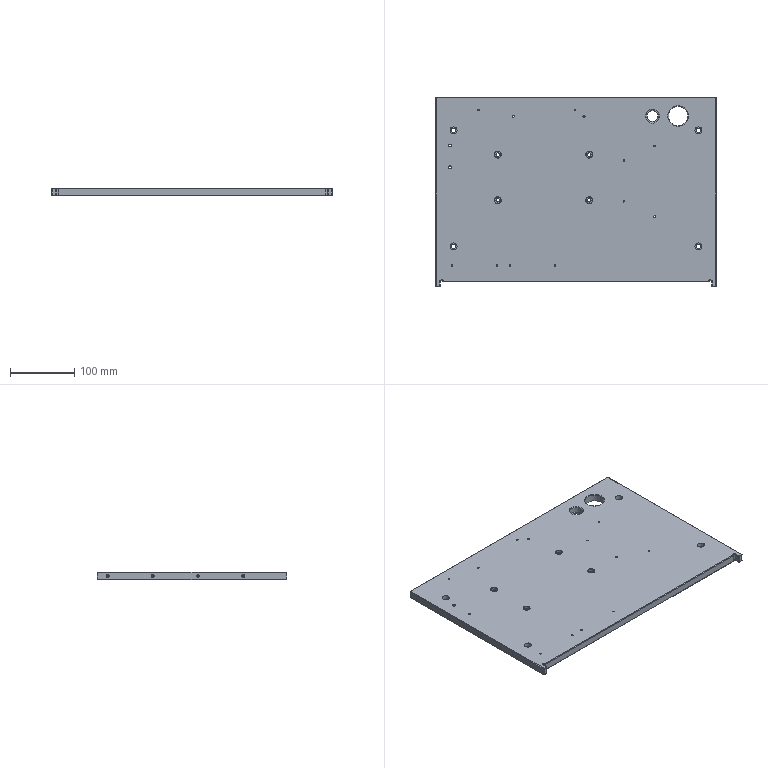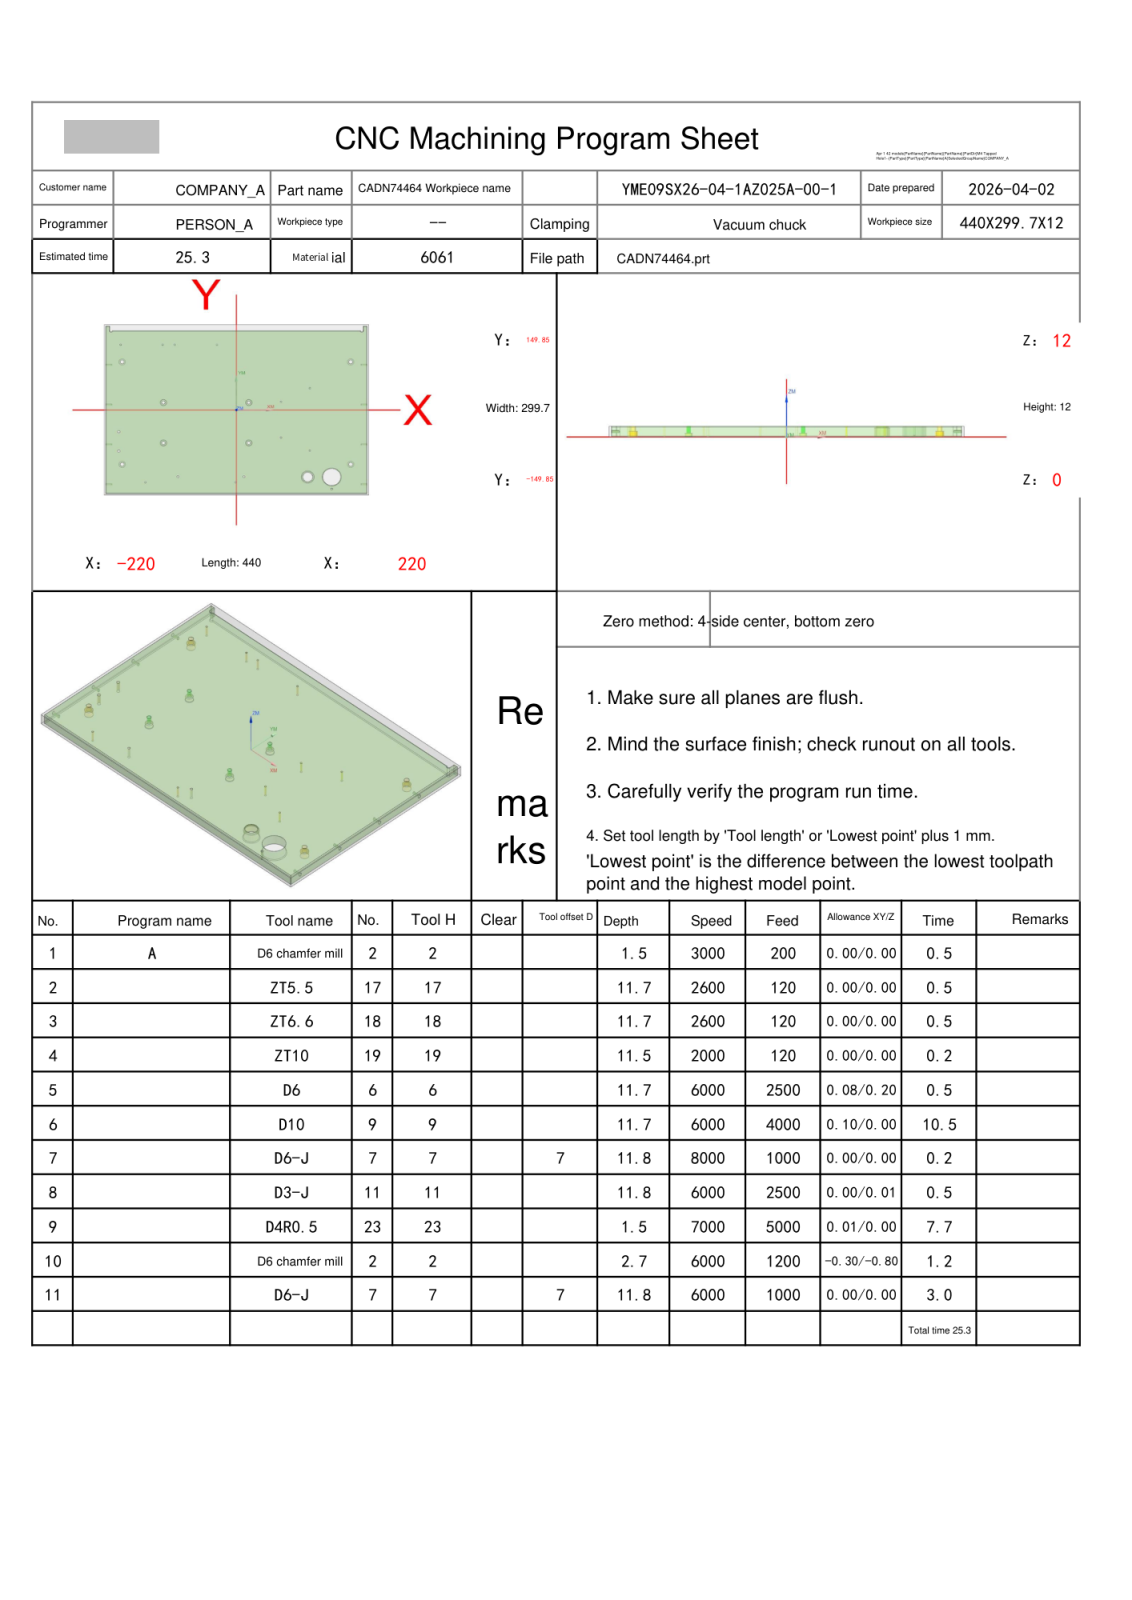NC program | NX | posted by the shop | part box 435 x 294.7 x 12 mm
Lines 1 to 895 of 24066:
%
O0001
(Machine time: 27.52 MIN)
(===Total Tool:9===)
(T2=D6 chamfer mill   D=6.   R=0.   D-  H02 Z=9.3   )
(T17=ZT5.5  D=5.5  DR_a=118 D-  H17 Z=0.3   )
(T18=ZT6.6  D=6.6  DR_a=118 D-  H18 Z=0.3   )
(T19=ZT10   D=10.  DR_a=118 D-  H19 Z=0.5   )
(T6=D6      D=6.   R=0.   D-  H06 Z=0.3   )
(T9=D10     D=10.  R=0.   D-  H09 Z=0.3   )
(T7=D6-J    D=6.   R=0.   D7  H07 Z=0.2   )
(T11=D3-J   D=3.   R=0.   D-  H11 Z=0.2   )
(T23=D4R0.5 D=4.   R=0.5  D-  H23 Z=10.5  )
G80 G90 G17 G49 G40
G91 G28 Z0
M01
N1 T02 M06
(D6 chamfer mill  D=6. R=0. H=02 ce=0.00 di=0.00)
G00 G90 G54 X-190. Y84.346 M03 S3000
G43 H02 Z32.
M08
G98 G81 X-190. Y84.346 Z10.5 R13. F200.
X-195.5 Y-38.35
Y-72.35
X-190. Y-95.654
X-97.5 Y-117.35
X-121.425 Y-58.109
Y12.891
X20.575
Y-58.109
X12.5 Y-117.35
X118.5 Y-117.85
X158.5 Y-138.85
Y-117.85
X190. Y-95.654
Y84.346
G80
G00 Z32.
G00 G90 X-151.5 Y-127.35 M03 S3000
Z32.
G98 G81 X-151.5 Y-127.35 Z11. R13. F200.
X-1.5
X74.218 Y-48.701
X121.901 Y-71.329
Y38.171
X74.218 Y14.299
X-32.5 Y114.35
X-102.5
X-122.5
X-192.5
G80
G00 Z32.
G91 G28 Z0.0
M05
M09
G91 G28 Z0.0
M01
N2 T17 M06
(ZT5.5 D=5.5 DR_a=118 H=17)
G00 G90 G54 X-121.425 Y12.891 M03 S2600
G43 H17 Z32.
M08
G98 G83 X-121.425 Y12.891 Z.3 R13. F120. Q1.5
Y-58.109
X20.575
Y12.891
G80
G00 Z32.
G91 G28 Z0.0
M05
M09
G91 G28 Z0.0
M01
N3 T18 M06
(ZT6.6 D=6.6 DR_a=118 H=18)
G00 G90 G54 X-190. Y84.346 M03 S2600
G43 H18 Z32.
M08
G98 G83 X-190. Y84.346 Z.3 R13. F120. Q1.5
Y-95.654
X190.
Y84.346
G80
G00 Z32.
G91 G28 Z0.0
M05
M09
G91 G28 Z0.0
M01
N4 T19 M06
(ZT10 D=10. DR_a=118 H=19)
G00 G90 G54 X118.5 Y-117.85 M03 S2000
G43 H19 Z32.
M08
G98 G83 X118.5 Y-117.85 Z.5 R13. F120. Q1.5
G80
G00 Z32.
G00 G90 X158.5 Y-117.85 M03 S1500
Z32.
G98 G83 X158.5 Y-117.85 Z.5 R13. F120. Q3.
G80
G00 Z32.
G91 G28 Z0.0
M05
M09
G91 G28 Z0.0
M01
N5 T06 M06
(D6  D=6. R=0. H=06 ce=0.08 di=0.20)
G00 G90 G54 X118.5 Y-117.85 M03 S6000
G43 H06 Z32.
M08
Z12.5
G03 X119.75 Y-119.1 I1.25 J0.0 F2250.
X121. Y-117.85 I0.0 J1.25
X121. Y-117.85 Z12.3 I-2.5 J0.0 F2500.
X121. Y-117.85 Z12.1 I-2.5 J0.0
X121. Y-117.85 Z11.9 I-2.5 J0.0
X121. Y-117.85 Z11.7 I-2.5 J0.0
X121. Y-117.85 Z11.5 I-2.5 J0.0
X121. Y-117.85 Z11.3 I-2.5 J0.0
X121. Y-117.85 Z11.1 I-2.5 J0.0
X121. Y-117.85 Z10.9 I-2.5 J0.0
X121. Y-117.85 Z10.7 I-2.5 J0.0
X121. Y-117.85 Z10.5 I-2.5 J0.0
X121. Y-117.85 Z10.3 I-2.5 J0.0
X121. Y-117.85 Z10.1 I-2.5 J0.0
X121. Y-117.85 Z9.9 I-2.5 J0.0
X121. Y-117.85 Z9.7 I-2.5 J0.0
X121. Y-117.85 Z9.5 I-2.5 J0.0
X121. Y-117.85 Z9.3 I-2.5 J0.0
X121. Y-117.85 Z9.1 I-2.5 J0.0
X121. Y-117.85 Z8.9 I-2.5 J0.0
X121. Y-117.85 Z8.7 I-2.5 J0.0
X121. Y-117.85 Z8.5 I-2.5 J0.0
X121. Y-117.85 Z8.3 I-2.5 J0.0
X121. Y-117.85 Z8.1 I-2.5 J0.0
X121. Y-117.85 Z7.9 I-2.5 J0.0
X121. Y-117.85 Z7.7 I-2.5 J0.0
X121. Y-117.85 Z7.5 I-2.5 J0.0
X121. Y-117.85 Z7.3 I-2.5 J0.0
X121. Y-117.85 Z7.1 I-2.5 J0.0
X121. Y-117.85 Z6.9 I-2.5 J0.0
X121. Y-117.85 Z6.7 I-2.5 J0.0
X121. Y-117.85 Z6.5 I-2.5 J0.0
X116. Y-117.85 Z6.4 I-2.5 J0.0
X118.465 Y-120.436 I2.589 J0.0
G01 X118.592 Y-120.439
G03 X121.231 Y-118.1 I0.0 J2.658
X121.251 Y-117.766 I-2.765 J.335
X118.923 Y-115.018 I-2.785 J0.0
X118.441 Y-114.978 I-.483 J-2.901
X115.564 Y-117.307 I0.0 J-2.94
X115.498 Y-117.937 I2.962 J-.63
X117.765 Y-120.868 I3.028 J0.0
X118.565 Y-120.97 I.8 J3.081
X121.608 Y-118.724 I0.0 J3.183
X121.753 Y-117.761 I-3.126 J.963
X119.584 Y-114.681 I-3.271 J0.0
X118.429 Y-114.481 I-1.154 J-3.226
X115.258 Y-116.609 I0.0 J-3.426
X114.997 Y-117.94 I3.252 J-1.331
X117.035 Y-121.129 I3.514 J0.0
X118.576 Y-121.468 I1.541 J3.33
X121.833 Y-119.489 I0.0 J3.669
X122.254 Y-117.759 I-3.335 J1.729
X120.375 Y-114.505 I-3.757 J0.0
X118.42 Y-113.982 I-1.955 J-3.388
X115.124 Y-115.788 I0.0 J-3.912
X114.495 Y-117.941 I3.37 J-2.153
X116.191 Y-121.211 I3.999 J0.0
X118.583 Y-121.968 I2.392 J3.397
X121.869 Y-120.357 I0.0 J4.154
X122.756 Y-117.76 I-3.355 J2.597
X121.259 Y-114.526 I-4.242 J0.0
X118.414 Y-113.481 I-2.846 J-3.352
X115.193 Y-114.884 I0.0 J-4.397
X113.993 Y-117.938 I3.285 J-3.054
X115.279 Y-121.081 I4.485 J0.0
X118.589 Y-122.47 I3.31 J3.252
X121.687 Y-121.283 I0.0 J4.64
X123.258 Y-117.764 I-3.157 J3.519
X122.188 Y-114.769 I-4.728 J0.0
X118.41 Y-112.98 I-3.778 J-3.093
X115.491 Y-113.948 I0.0 J-4.883
X113.476 Y-117.965 I2.995 J-4.017
X114.38 Y-120.836 I5.011 J0.0
X118.546 Y-123.007 I4.167 J2.913
X121.27 Y-122.215 I0.0 J5.084
X123.67 Y-117.85 I-2.77 J4.365
X118.5 Y-112.68 I-5.17 J0.0
X113.33 Y-117.85 I0.0 J-5.17
X118.5 Y-123.02 I5.17 J0.0
X121.679 Y-121.927 I0.0 J5.17
X122.674 Y-119.889 I-1.589 J2.039
X120.089 Y-117.304 I-2.585 J0.0
X118.5 Y-117.85 I0.0 J-2.585
X119.75 Y-119.1 I1.25 J0.0 F2250.
X121. Y-117.85 I0.0 J1.25
X121. Y-117.85 Z6.2 I-2.5 J0.0 F2500.
X121. Y-117.85 Z6. I-2.5 J0.0
X121. Y-117.85 Z5.8 I-2.5 J0.0
X121. Y-117.85 Z5.6 I-2.5 J0.0
X121. Y-117.85 Z5.4 I-2.5 J0.0
X121. Y-117.85 Z5.2 I-2.5 J0.0
X121. Y-117.85 Z5. I-2.5 J0.0
X121. Y-117.85 Z4.8 I-2.5 J0.0
X121. Y-117.85 Z4.6 I-2.5 J0.0
X121. Y-117.85 Z4.4 I-2.5 J0.0
X121. Y-117.85 Z4.2 I-2.5 J0.0
X121. Y-117.85 Z4. I-2.5 J0.0
X121. Y-117.85 Z3.8 I-2.5 J0.0
X121. Y-117.85 Z3.6 I-2.5 J0.0
X121. Y-117.85 Z3.4 I-2.5 J0.0
X121. Y-117.85 Z3.2 I-2.5 J0.0
X121. Y-117.85 Z3. I-2.5 J0.0
X121. Y-117.85 Z2.8 I-2.5 J0.0
X121. Y-117.85 Z2.6 I-2.5 J0.0
X121. Y-117.85 Z2.4 I-2.5 J0.0
X121. Y-117.85 Z2.2 I-2.5 J0.0
X121. Y-117.85 Z2. I-2.5 J0.0
X121. Y-117.85 Z1.8 I-2.5 J0.0
X121. Y-117.85 Z1.6 I-2.5 J0.0
X121. Y-117.85 Z1.4 I-2.5 J0.0
X121. Y-117.85 Z1.2 I-2.5 J0.0
X121. Y-117.85 Z1. I-2.5 J0.0
X121. Y-117.85 Z.8 I-2.5 J0.0
X121. Y-117.85 Z.6 I-2.5 J0.0
X121. Y-117.85 Z.4 I-2.5 J0.0
X116. Y-117.85 Z.3 I-2.5 J0.0
X118.465 Y-120.436 I2.589 J0.0
G01 X118.592 Y-120.439
G03 X121.231 Y-118.1 I0.0 J2.658
X121.251 Y-117.766 I-2.765 J.335
X118.923 Y-115.018 I-2.785 J0.0
X118.441 Y-114.978 I-.483 J-2.901
X115.564 Y-117.307 I0.0 J-2.94
X115.498 Y-117.937 I2.962 J-.63
X117.765 Y-120.868 I3.028 J0.0
X118.565 Y-120.97 I.8 J3.081
X121.608 Y-118.724 I0.0 J3.183
X121.753 Y-117.761 I-3.126 J.963
X119.584 Y-114.681 I-3.271 J0.0
X118.429 Y-114.481 I-1.154 J-3.226
X115.258 Y-116.609 I0.0 J-3.426
X114.997 Y-117.94 I3.252 J-1.331
X117.035 Y-121.129 I3.514 J0.0
X118.576 Y-121.468 I1.541 J3.33
X121.833 Y-119.489 I0.0 J3.669
X122.254 Y-117.759 I-3.335 J1.729
X120.375 Y-114.505 I-3.757 J0.0
X118.42 Y-113.982 I-1.955 J-3.388
X115.124 Y-115.788 I0.0 J-3.912
X114.495 Y-117.941 I3.37 J-2.153
X116.191 Y-121.211 I3.999 J0.0
X118.583 Y-121.968 I2.392 J3.397
X121.869 Y-120.357 I0.0 J4.154
X122.756 Y-117.76 I-3.355 J2.597
X121.259 Y-114.526 I-4.242 J0.0
X118.414 Y-113.481 I-2.846 J-3.352
X115.193 Y-114.884 I0.0 J-4.397
X113.993 Y-117.938 I3.285 J-3.054
X115.279 Y-121.081 I4.485 J0.0
X118.589 Y-122.47 I3.31 J3.252
X121.687 Y-121.283 I0.0 J4.64
X123.258 Y-117.764 I-3.157 J3.519
X122.188 Y-114.769 I-4.728 J0.0
X118.41 Y-112.98 I-3.778 J-3.093
X115.491 Y-113.948 I0.0 J-4.883
X113.476 Y-117.965 I2.995 J-4.017
X114.38 Y-120.836 I5.011 J0.0
X118.546 Y-123.007 I4.167 J2.913
X121.27 Y-122.215 I0.0 J5.084
X123.67 Y-117.85 I-2.77 J4.365
X118.5 Y-112.68 I-5.17 J0.0
X113.33 Y-117.85 I0.0 J-5.17
X118.5 Y-123.02 I5.17 J0.0
X121.679 Y-121.927 I0.0 J5.17
X122.674 Y-119.889 I-1.589 J2.039
X120.089 Y-117.304 I-2.585 J0.0
X118.5 Y-117.85 I0.0 J-2.585
G00 Z32.
G91 G28 Z0.0
M05
M09
G91 G28 Z0.0
M01
N6 T09 M06
(D10  D=10. R=0. H=09 ce=0.10 di=0.30)
G00 G90 G54 X158.5 Y-117.85 M03 S6000
G43 H09 Z32.
M08
Z12.5
G03 X160.5 Y-119.85 I2. J0.0 F2700.
X162.5 Y-117.85 I0.0 J2.
X162.5 Y-117.85 Z12.3 I-4. J0.0 F3000.
X162.5 Y-117.85 Z12.1 I-4. J0.0
X162.5 Y-117.85 Z11.9 I-4. J0.0
X162.5 Y-117.85 Z11.7 I-4. J0.0
X162.5 Y-117.85 Z11.5 I-4. J0.0
X162.5 Y-117.85 Z11.3 I-4. J0.0
X162.5 Y-117.85 Z11.1 I-4. J0.0
X162.5 Y-117.85 Z10.9 I-4. J0.0
X162.5 Y-117.85 Z10.7 I-4. J0.0
X162.5 Y-117.85 Z10.5 I-4. J0.0
X162.5 Y-117.85 Z10.3 I-4. J0.0
X162.5 Y-117.85 Z10.1 I-4. J0.0
X162.5 Y-117.85 Z9.9 I-4. J0.0
X162.5 Y-117.85 Z9.7 I-4. J0.0
X162.5 Y-117.85 Z9.5 I-4. J0.0
X162.5 Y-117.85 Z9.3 I-4. J0.0
X162.5 Y-117.85 Z9.1 I-4. J0.0
X162.5 Y-117.85 Z8.9 I-4. J0.0
X162.5 Y-117.85 Z8.7 I-4. J0.0
X162.5 Y-117.85 Z8.5 I-4. J0.0
X162.5 Y-117.85 Z8.3 I-4. J0.0
X162.5 Y-117.85 Z8.1 I-4. J0.0
X162.5 Y-117.85 Z7.9 I-4. J0.0
X162.5 Y-117.85 Z7.7 I-4. J0.0
X162.5 Y-117.85 Z7.5 I-4. J0.0
X162.5 Y-117.85 Z7.3 I-4. J0.0
X162.5 Y-117.85 Z7.1 I-4. J0.0
X162.5 Y-117.85 Z6.9 I-4. J0.0
X162.5 Y-117.85 Z6.7 I-4. J0.0
X162.5 Y-117.85 Z6.5 I-4. J0.0
X162.5 Y-117.85 Z6.3 I-4. J0.0
X162.5 Y-117.85 Z6.1 I-4. J0.0
X162.5 Y-117.85 Z5.9 I-4. J0.0
X162.5 Y-117.85 Z5.7 I-4. J0.0
X162.5 Y-117.85 Z5.5 I-4. J0.0
X162.5 Y-117.85 Z5.3 I-4. J0.0
X162.5 Y-117.85 Z5.1 I-4. J0.0
X162.5 Y-117.85 Z4.9 I-4. J0.0
X162.5 Y-117.85 Z4.7 I-4. J0.0
X162.5 Y-117.85 Z4.5 I-4. J0.0
X162.5 Y-117.85 Z4.3 I-4. J0.0
X162.5 Y-117.85 Z4.1 I-4. J0.0
X162.5 Y-117.85 Z3.9 I-4. J0.0
X162.5 Y-117.85 Z3.7 I-4. J0.0
X162.5 Y-117.85 Z3.5 I-4. J0.0
X162.5 Y-117.85 Z3.3 I-4. J0.0
X162.5 Y-117.85 Z3.1 I-4. J0.0
X162.5 Y-117.85 Z2.9 I-4. J0.0
X162.5 Y-117.85 Z2.7 I-4. J0.0
X162.5 Y-117.85 Z2.5 I-4. J0.0
X162.5 Y-117.85 Z2.3 I-4. J0.0
X162.5 Y-117.85 Z2.1 I-4. J0.0
X162.5 Y-117.85 Z1.9 I-4. J0.0
X162.5 Y-117.85 Z1.7 I-4. J0.0
X162.5 Y-117.85 Z1.5 I-4. J0.0
X162.5 Y-117.85 Z1.3 I-4. J0.0
X162.5 Y-117.85 Z1.1 I-4. J0.0
X162.5 Y-117.85 Z.9 I-4. J0.0
X162.5 Y-117.85 Z.7 I-4. J0.0
X162.5 Y-117.85 Z.5 I-4. J0.0
X162.5 Y-117.85 Z.3 I-4. J0.0
X158.523 Y-113.764 I-4.088 J0.0
G01 X158.41 Y-113.762
G03 X154.26 Y-117.628 I0.0 J-4.161
X154.249 Y-117.933 I4.279 J-.305
X158.124 Y-122.202 I4.29 J0.0
X158.554 Y-122.223 I.43 J4.426
X162.967 Y-118.32 I0.0 J4.446
X163.001 Y-117.766 I-4.502 J.554
X159.135 Y-113.28 I-4.536 J0.0
X158.442 Y-113.228 I-.693 J-4.641
X153.821 Y-117.109 I0.0 J-4.692
X153.749 Y-117.936 I4.709 J-.827
X157.582 Y-122.622 I4.781 J0.0
X158.561 Y-122.721 I.979 J4.84
X163.374 Y-118.886 I0.0 J4.938
X163.502 Y-117.762 I-4.9 J1.124
X159.724 Y-112.893 I-5.027 J0.0
X158.435 Y-112.73 I-1.289 J-5.021
X153.449 Y-116.497 I0.0 J-5.184
X153.248 Y-117.939 I5.072 J-1.442
X156.948 Y-122.972 I5.273 J0.0
X158.568 Y-123.219 I1.619 J5.183
X163.707 Y-119.542 I0.0 J5.43
X164.002 Y-117.76 I-5.224 J1.782
X160.4 Y-112.585 I-5.519 J0.0
X158.429 Y-112.232 I-1.97 J-5.323
X153.159 Y-115.8 I0.0 J-5.676
X152.747 Y-117.94 I5.353 J-2.141
X156.233 Y-123.236 I5.765 J0.0
X158.574 Y-123.718 I2.34 J5.439
X163.951 Y-120.277 I0.0 J5.922
X164.504 Y-117.759 I-5.458 J2.518
X161.151 Y-112.368 I-6.011 J0.0
X158.424 Y-111.732 I-2.728 J-5.531
X152.965 Y-115.03 I0.0 J-6.167
X152.246 Y-117.941 I5.538 J-2.912
X155.448 Y-123.402 I6.257 J0.0
X158.579 Y-124.218 I3.131 J5.597
X164.093 Y-121.079 I0.0 J6.413
X165.005 Y-117.759 I-5.591 J3.32
X161.967 Y-112.256 I-6.502 J0.0
X158.419 Y-111.232 I-3.548 J-5.635
X152.877 Y-114.199 I0.0 J-6.659
X151.745 Y-117.941 I5.616 J-3.742
X154.606 Y-123.457 I6.748 J0.0
X158.583 Y-124.718 I3.977 J5.645
X164.123 Y-121.935 I0.0 J6.905
X165.506 Y-117.76 I-5.611 J4.176
X162.832 Y-112.259 I-6.994 J0.0
X158.415 Y-110.732 I-4.417 J-5.624
X152.908 Y-113.322 I0.0 J-7.151
X151.244 Y-117.94 I5.576 J-4.618
X153.722 Y-123.394 I7.24 J0.0
X158.587 Y-125.218 I4.865 J5.572
X164.03 Y-122.829 I0.0 J7.397
X166.007 Y-117.761 I-5.509 J5.068
X163.731 Y-112.386 I-7.486 J0.0
X158.412 Y-110.231 I-5.319 J-5.488
X153.064 Y-112.414 I0.0 J-7.643
X150.743 Y-117.937 I5.41 J-5.523
X152.812 Y-123.202 I7.732 J0.0
X158.589 Y-125.719 I5.777 J5.371
X163.808 Y-123.746 I0.0 J7.888
X166.508 Y-117.764 I-5.278 J5.982
X164.647 Y-112.643 I-7.977 J0.0
X158.41 Y-109.73 I-6.237 J-5.221
X153.353 Y-111.494 I0.0 J-8.134
X150.242 Y-117.934 I5.113 J-6.441
X151.894 Y-122.878 I8.223 J0.0
X158.591 Y-126.22 I6.697 J5.038
X163.452 Y-124.666 I0.0 J8.38
X167.008 Y-117.768 I-4.913 J6.898
X165.563 Y-113.036 I-8.469 J0.0
X158.409 Y-109.229 I-7.154 J-4.819
X153.778 Y-110.578 I0.0 J-8.626
X149.742 Y-117.93 I4.679 J-7.352
X150.985 Y-122.416 I8.715 J0.0
X158.591 Y-126.721 I7.606 J4.567
X162.958 Y-125.572 I0.0 J8.872
X167.508 Y-117.772 I-4.411 J7.8
X166.46 Y-113.566 I-8.961 J0.0
X158.409 Y-108.728 I-8.051 J-4.28
X154.34 Y-109.686 I0.0 J-9.118
X149.242 Y-117.925 I4.108 J-8.239
X150.105 Y-121.818 I9.207 J0.0
X158.591 Y-127.223 I8.486 J3.958
X162.327 Y-126.445 I0.0 J9.363
X168.008 Y-117.777 I-3.772 J8.668
X167.318 Y-114.233 I-9.453 J0.0
X158.41 Y-108.227 I-8.908 J-3.603
X155.04 Y-108.837 I0.0 J-9.609
X148.717 Y-117.957 I3.415 J-9.12
X149.274 Y-121.205 I9.738 J0.0
X158.527 Y-127.746 I9.252 J3.273
X161.559 Y-127.265 I0.0 J9.814
X168.4 Y-117.85 I-3.059 J9.415
X158.5 Y-107.95 I-9.9 J0.0
X148.6 Y-117.85 I0.0 J-9.9
X158.5 Y-127.75 I9.9 J0.0
X162.031 Y-127.099 I0.0 J9.9
X165.215 Y-122.475 I-1.765 J4.625
X160.265 Y-117.525 I-4.95 J0.0
X158.5 Y-117.85 I0.0 J-4.95
G00 Z32.
G00 G90 X0.0 Y-152.45 M03 S6000
Z32.
Z12.5
G01 X-216.5 Z12.431 F4000.
G02 X-222.6 Y-146.35 Z12.428 I0.0 J6.1
G01 Y146.35 Z12.334
G02 X-216.5 Y152.45 Z12.331 I6.1 J0.0
G01 X-211.5 Z12.329
G02 X-205.4 Y146.35 Z12.326 I0.0 J-6.1
G01 Y144.45
X205.4 Z12.194
Y146.35
G02 X211.5 Y152.45 Z12.191 I6.1 J0.0
G01 X216.5 Z12.189
G02 X222.6 Y146.35 Z12.186 I0.0 J-6.1
G01 Y-146.35 Z12.092
G02 X216.5 Y-152.45 Z12.089 I-6.1 J0.0
G01 X-216.5 Z11.951
G02 X-222.6 Y-146.35 Z11.948 I0.0 J6.1
G01 Y146.35 Z11.854
G02 X-216.5 Y152.45 Z11.851 I6.1 J0.0
G01 X-211.5 Z11.849
G02 X-205.4 Y146.35 Z11.846 I0.0 J-6.1
G01 Y144.45
X205.4 Z11.714
Y146.35
G02 X211.5 Y152.45 Z11.711 I6.1 J0.0
G01 X216.5 Z11.709
G02 X222.6 Y146.35 Z11.706 I0.0 J-6.1
G01 Y-146.35 Z11.612
G02 X216.5 Y-152.45 Z11.609 I-6.1 J0.0
G01 X-216.5 Z11.471
G02 X-222.6 Y-146.35 Z11.468 I0.0 J6.1
G01 Y146.35 Z11.374
G02 X-216.5 Y152.45 Z11.371 I6.1 J0.0
G01 X-211.5 Z11.369
G02 X-205.4 Y146.35 Z11.366 I0.0 J-6.1
G01 Y144.45
X205.4 Z11.234
Y146.35
G02 X211.5 Y152.45 Z11.231 I6.1 J0.0
G01 X216.5 Z11.229
G02 X222.6 Y146.35 Z11.226 I0.0 J-6.1
G01 Y-146.35 Z11.132
G02 X216.5 Y-152.45 Z11.129 I-6.1 J0.0
G01 X-216.5 Z10.991
G02 X-222.6 Y-146.35 Z10.988 I0.0 J6.1
G01 Y146.35 Z10.894
G02 X-216.5 Y152.45 Z10.891 I6.1 J0.0
G01 X-211.5 Z10.889
G02 X-205.4 Y146.35 Z10.886 I0.0 J-6.1
G01 Y144.45
X205.4 Z10.754
Y146.35
G02 X211.5 Y152.45 Z10.751 I6.1 J0.0
G01 X216.5 Z10.749
G02 X222.6 Y146.35 Z10.746 I0.0 J-6.1
G01 Y-146.35 Z10.652
G02 X216.5 Y-152.45 Z10.649 I-6.1 J0.0
G01 X-216.5 Z10.511
G02 X-222.6 Y-146.35 Z10.508 I0.0 J6.1
G01 Y146.35 Z10.414
G02 X-216.5 Y152.45 Z10.411 I6.1 J0.0
G01 X-211.5 Z10.409
G02 X-205.4 Y146.35 Z10.406 I0.0 J-6.1
G01 Y144.45
X205.4 Z10.274
Y146.35
G02 X211.5 Y152.45 Z10.271 I6.1 J0.0
G01 X216.5 Z10.269
G02 X222.6 Y146.35 Z10.266 I0.0 J-6.1
G01 Y-146.35 Z10.172
G02 X216.5 Y-152.45 Z10.169 I-6.1 J0.0
G01 X-216.5 Z10.031
G02 X-222.6 Y-146.35 Z10.028 I0.0 J6.1
G01 Y146.35 Z9.934
G02 X-216.5 Y152.45 Z9.931 I6.1 J0.0
G01 X-211.5 Z9.929
G02 X-205.4 Y146.35 Z9.926 I0.0 J-6.1
G01 Y144.45
X205.4 Z9.794
Y146.35
G02 X211.5 Y152.45 Z9.791 I6.1 J0.0
G01 X216.5 Z9.789
G02 X222.6 Y146.35 Z9.786 I0.0 J-6.1
G01 Y-146.35 Z9.692
G02 X216.5 Y-152.45 Z9.689 I-6.1 J0.0
G01 X-216.5 Z9.551
G02 X-222.6 Y-146.35 Z9.548 I0.0 J6.1
G01 Y146.35 Z9.454
G02 X-216.5 Y152.45 Z9.451 I6.1 J0.0
G01 X-211.5 Z9.449
G02 X-205.4 Y146.35 Z9.446 I0.0 J-6.1
G01 Y144.45
X205.4 Z9.314
Y146.35
G02 X211.5 Y152.45 Z9.311 I6.1 J0.0
G01 X216.5 Z9.309
G02 X222.6 Y146.35 Z9.306 I0.0 J-6.1
G01 Y-146.35 Z9.212
G02 X216.5 Y-152.45 Z9.209 I-6.1 J0.0
G01 X-216.5 Z9.071
G02 X-222.6 Y-146.35 Z9.068 I0.0 J6.1
G01 Y146.35 Z8.974
G02 X-216.5 Y152.45 Z8.971 I6.1 J0.0
G01 X-211.5 Z8.969
G02 X-205.4 Y146.35 Z8.966 I0.0 J-6.1
G01 Y144.45
X205.4 Z8.834
Y146.35
G02 X211.5 Y152.45 Z8.831 I6.1 J0.0
G01 X216.5 Z8.829
G02 X222.6 Y146.35 Z8.826 I0.0 J-6.1
G01 Y-146.35 Z8.732
G02 X216.5 Y-152.45 Z8.729 I-6.1 J0.0
G01 X-216.5 Z8.591
G02 X-222.6 Y-146.35 Z8.588 I0.0 J6.1
G01 Y146.35 Z8.494
G02 X-216.5 Y152.45 Z8.491 I6.1 J0.0
G01 X-211.5 Z8.489
G02 X-205.4 Y146.35 Z8.486 I0.0 J-6.1
G01 Y144.45
X205.4 Z8.354
Y146.35
G02 X211.5 Y152.45 Z8.351 I6.1 J0.0
G01 X216.5 Z8.349
G02 X222.6 Y146.35 Z8.346 I0.0 J-6.1
G01 Y-146.35 Z8.252
G02 X216.5 Y-152.45 Z8.249 I-6.1 J0.0
G01 X-216.5 Z8.111
G02 X-222.6 Y-146.35 Z8.108 I0.0 J6.1
G01 Y146.35 Z8.014
G02 X-216.5 Y152.45 Z8.011 I6.1 J0.0
G01 X-211.5 Z8.009
G02 X-205.4 Y146.35 Z8.006 I0.0 J-6.1
G01 Y144.45
X205.4 Z7.874
Y146.35
G02 X211.5 Y152.45 Z7.871 I6.1 J0.0
G01 X216.5 Z7.869
G02 X222.6 Y146.35 Z7.866 I0.0 J-6.1
G01 Y-146.35 Z7.772
G02 X216.5 Y-152.45 Z7.769 I-6.1 J0.0
G01 X-216.5 Z7.631
G02 X-222.6 Y-146.35 Z7.628 I0.0 J6.1
G01 Y146.35 Z7.534
G02 X-216.5 Y152.45 Z7.531 I6.1 J0.0
G01 X-211.5 Z7.529
G02 X-205.4 Y146.35 Z7.526 I0.0 J-6.1
G01 Y144.45
X205.4 Z7.394
Y146.35
G02 X211.5 Y152.45 Z7.391 I6.1 J0.0
G01 X216.5 Z7.389
G02 X222.6 Y146.35 Z7.386 I0.0 J-6.1
G01 Y-146.35 Z7.292
G02 X216.5 Y-152.45 Z7.289 I-6.1 J0.0
G01 X-216.5 Z7.151
G02 X-222.6 Y-146.35 Z7.148 I0.0 J6.1
G01 Y146.35 Z7.054
G02 X-216.5 Y152.45 Z7.051 I6.1 J0.0
G01 X-211.5 Z7.049
G02 X-205.4 Y146.35 Z7.046 I0.0 J-6.1
G01 Y144.45
X205.4 Z6.914
Y146.35
G02 X211.5 Y152.45 Z6.911 I6.1 J0.0
G01 X216.5 Z6.909
G02 X222.6 Y146.35 Z6.906 I0.0 J-6.1
G01 Y-146.35 Z6.812
G02 X216.5 Y-152.45 Z6.809 I-6.1 J0.0
G01 X-216.5 Z6.671
G02 X-222.6 Y-146.35 Z6.668 I0.0 J6.1
G01 Y146.35 Z6.574
G02 X-216.5 Y152.45 Z6.571 I6.1 J0.0
G01 X-211.5 Z6.569
G02 X-205.4 Y146.35 Z6.566 I0.0 J-6.1
G01 Y144.45
X205.4 Z6.434
Y146.35
G02 X211.5 Y152.45 Z6.431 I6.1 J0.0
G01 X216.5 Z6.429
G02 X222.6 Y146.35 Z6.426 I0.0 J-6.1
G01 Y-146.35 Z6.332
G02 X216.5 Y-152.45 Z6.329 I-6.1 J0.0
G01 X-216.5 Z6.191
G02 X-222.6 Y-146.35 Z6.188 I0.0 J6.1
G01 Y146.35 Z6.094
G02 X-216.5 Y152.45 Z6.091 I6.1 J0.0
G01 X-211.5 Z6.089
G02 X-205.4 Y146.35 Z6.086 I0.0 J-6.1
G01 Y144.45
X205.4 Z5.954
Y146.35
G02 X211.5 Y152.45 Z5.951 I6.1 J0.0
G01 X216.5 Z5.949
G02 X222.6 Y146.35 Z5.946 I0.0 J-6.1
G01 Y-146.35 Z5.852
G02 X216.5 Y-152.45 Z5.849 I-6.1 J0.0
G01 X-216.5 Z5.711
G02 X-222.6 Y-146.35 Z5.708 I0.0 J6.1
G01 Y146.35 Z5.614
G02 X-216.5 Y152.45 Z5.611 I6.1 J0.0
G01 X-211.5 Z5.609
G02 X-205.4 Y146.35 Z5.606 I0.0 J-6.1
G01 Y144.45
X205.4 Z5.474
Y146.35
G02 X211.5 Y152.45 Z5.471 I6.1 J0.0
G01 X216.5 Z5.469
G02 X222.6 Y146.35 Z5.466 I0.0 J-6.1
G01 Y-146.35 Z5.372
G02 X216.5 Y-152.45 Z5.369 I-6.1 J0.0
G01 X-216.5 Z5.231
G02 X-222.6 Y-146.35 Z5.228 I0.0 J6.1
G01 Y146.35 Z5.134
G02 X-216.5 Y152.45 Z5.131 I6.1 J0.0
G01 X-211.5 Z5.129
G02 X-205.4 Y146.35 Z5.126 I0.0 J-6.1
G01 Y144.45
X205.4 Z4.994
Y146.35
G02 X211.5 Y152.45 Z4.991 I6.1 J0.0
G01 X216.5 Z4.989
G02 X222.6 Y146.35 Z4.986 I0.0 J-6.1
G01 Y-146.35 Z4.892
G02 X216.5 Y-152.45 Z4.889 I-6.1 J0.0
G01 X-216.5 Z4.751
G02 X-222.6 Y-146.35 Z4.748 I0.0 J6.1
G01 Y146.35 Z4.654
G02 X-216.5 Y152.45 Z4.651 I6.1 J0.0
G01 X-211.5 Z4.649
G02 X-205.4 Y146.35 Z4.646 I0.0 J-6.1
G01 Y144.45
X205.4 Z4.514
Y146.35
G02 X211.5 Y152.45 Z4.511 I6.1 J0.0
G01 X216.5 Z4.509
G02 X222.6 Y146.35 Z4.506 I0.0 J-6.1
G01 Y-146.35 Z4.412
G02 X216.5 Y-152.45 Z4.409 I-6.1 J0.0
G01 X-216.5 Z4.271
G02 X-222.6 Y-146.35 Z4.268 I0.0 J6.1
G01 Y146.35 Z4.174
G02 X-216.5 Y152.45 Z4.171 I6.1 J0.0
G01 X-211.5 Z4.169
G02 X-205.4 Y146.35 Z4.166 I0.0 J-6.1
G01 Y144.45
X205.4 Z4.034
Y146.35
G02 X211.5 Y152.45 Z4.031 I6.1 J0.0
G01 X216.5 Z4.029
G02 X222.6 Y146.35 Z4.026 I0.0 J-6.1
G01 Y-146.35 Z3.932
G02 X216.5 Y-152.45 Z3.929 I-6.1 J0.0
G01 X-216.5 Z3.791
G02 X-222.6 Y-146.35 Z3.788 I0.0 J6.1
G01 Y146.35 Z3.694
G02 X-216.5 Y152.45 Z3.691 I6.1 J0.0
G01 X-211.5 Z3.689
G02 X-205.4 Y146.35 Z3.686 I0.0 J-6.1
G01 Y144.45
X205.4 Z3.554
Y146.35
G02 X211.5 Y152.45 Z3.551 I6.1 J0.0
G01 X216.5 Z3.549
G02 X222.6 Y146.35 Z3.546 I0.0 J-6.1
G01 Y-146.35 Z3.452
G02 X216.5 Y-152.45 Z3.449 I-6.1 J0.0
G01 X-216.5 Z3.311
G02 X-222.6 Y-146.35 Z3.308 I0.0 J6.1
G01 Y146.35 Z3.214
G02 X-216.5 Y152.45 Z3.211 I6.1 J0.0
G01 X-211.5 Z3.209
G02 X-205.4 Y146.35 Z3.206 I0.0 J-6.1
G01 Y144.45
X205.4 Z3.074
Y146.35
G02 X211.5 Y152.45 Z3.071 I6.1 J0.0
G01 X216.5 Z3.069
G02 X222.6 Y146.35 Z3.066 I0.0 J-6.1
G01 Y-146.35 Z2.972
G02 X216.5 Y-152.45 Z2.969 I-6.1 J0.0
G01 X-216.5 Z2.831
G02 X-222.6 Y-146.35 Z2.828 I0.0 J6.1
G01 Y146.35 Z2.734
G02 X-216.5 Y152.45 Z2.731 I6.1 J0.0
G01 X-211.5 Z2.729
G02 X-205.4 Y146.35 Z2.726 I0.0 J-6.1
G01 Y144.45
X205.4 Z2.594
Y146.35
G02 X211.5 Y152.45 Z2.591 I6.1 J0.0
G01 X216.5 Z2.589
G02 X222.6 Y146.35 Z2.586 I0.0 J-6.1
G01 Y-146.35 Z2.492
G02 X216.5 Y-152.45 Z2.489 I-6.1 J0.0
G01 X-216.5 Z2.351
G02 X-222.6 Y-146.35 Z2.348 I0.0 J6.1
G01 Y146.35 Z2.254
G02 X-216.5 Y152.45 Z2.251 I6.1 J0.0
G01 X-211.5 Z2.249
G02 X-205.4 Y146.35 Z2.246 I0.0 J-6.1
G01 Y144.45
X205.4 Z2.114
Y146.35
G02 X211.5 Y152.45 Z2.111 I6.1 J0.0
G01 X216.5 Z2.109
G02 X222.6 Y146.35 Z2.106 I0.0 J-6.1
G01 Y-146.35 Z2.012
G02 X216.5 Y-152.45 Z2.009 I-6.1 J0.0
G01 X-216.5 Z1.871
G02 X-222.6 Y-146.35 Z1.868 I0.0 J6.1
G01 Y146.35 Z1.774
G02 X-216.5 Y152.45 Z1.771 I6.1 J0.0
G01 X-211.5 Z1.769
G02 X-205.4 Y146.35 Z1.766 I0.0 J-6.1
G01 Y144.45
X205.4 Z1.634
Y146.35
G02 X211.5 Y152.45 Z1.631 I6.1 J0.0
G01 X216.5 Z1.629
G02 X222.6 Y146.35 Z1.626 I0.0 J-6.1
G01 Y-146.35 Z1.532
G02 X216.5 Y-152.45 Z1.529 I-6.1 J0.0
G01 X-216.5 Z1.391
G02 X-222.6 Y-146.35 Z1.388 I0.0 J6.1
G01 Y146.35 Z1.294
G02 X-216.5 Y152.45 Z1.291 I6.1 J0.0
G01 X-211.5 Z1.289
G02 X-205.4 Y146.35 Z1.286 I0.0 J-6.1
G01 Y144.45
X205.4 Z1.154
Y146.35
G02 X211.5 Y152.45 Z1.151 I6.1 J0.0
G01 X216.5 Z1.149
G02 X222.6 Y146.35 Z1.146 I0.0 J-6.1
G01 Y-146.35 Z1.052
G02 X216.5 Y-152.45 Z1.049 I-6.1 J0.0
G01 X-216.5 Z.911
G02 X-222.6 Y-146.35 Z.908 I0.0 J6.1
G01 Y146.35 Z.814
G02 X-216.5 Y152.45 Z.811 I6.1 J0.0
G01 X-211.5 Z.809
G02 X-205.4 Y146.35 Z.806 I0.0 J-6.1
G01 Y144.45
X205.4 Z.674
Y146.35
G02 X211.5 Y152.45 Z.671 I6.1 J0.0
G01 X216.5 Z.669
G02 X222.6 Y146.35 Z.666 I0.0 J-6.1
G01 Y-146.35 Z.572
G02 X216.5 Y-152.45 Z.569 I-6.1 J0.0
G01 X0.0 Z.5
X-216.5
G02 X-222.6 Y-146.35 I0.0 J6.1
G01 Y146.35
G02 X-216.5 Y152.45 I6.1 J0.0
G01 X-211.5
G02 X-205.4 Y146.35 I0.0 J-6.1
G01 Y144.45
X205.4
Y146.35
G02 X211.5 Y152.45 I6.1 J0.0
G01 X216.5
G02 X222.6 Y146.35 I0.0 J-6.1
G01 Y-146.35
G02 X216.5 Y-152.45 I-6.1 J0.0
G01 X0.0
X-.5
Z1.5
G00 Z32.
G91 G28 Z0.0
M05
M09
G91 G28 Z0.0
M01
N7 T07 M06
(D6-J  D=6. R=0. H=07 ce=0.00 di=0.00)
G00 G90 G54 X157.6 Y-128.713 M03 S8000
G43 H07 Z22.
M08
Z1.7
G01 Z.2 F1000.
G41 D07
Y-128.95
G03 X158.5 Y-129.85 I.9 J0.0
X170.5 Y-117.85 I0.0 J12.
X158.5 Y-105.85 I-12. J0.0
X146.5 Y-117.85 I0.0 J-12.
X158.5 Y-129.85 I12. J0.0
X158.9 Y-129.843 I0.0 J12.
X159.77 Y-128.944 I-.03 J.9
G01 X159.769 Y-128.914
X159.768 Y-128.877
G40 X159.762 Y-128.677
Z1.7
G00 Z22.
G00 G90 X122.035 Y-118.835 M03 S6000
Z32.
Z6.85
G41 D07
G01 X122.517 Y-118.969 F720.
X122.626 Y-118.974
G03 X123.75 Y-117.85 I0.0 J1.124
X118.5 Y-112.6 I-5.25 J0.0 F800.
X113.25 Y-117.85 I0.0 J-5.25
X118.5 Y-123.1 I5.25 J0.0
X123.75 Y-117.85 I0.0 J5.25
X123.726 Y-117.351 I-5.25 J0.0
X122.607 Y-116.334 I-1.119 J-.107
X122.393 Y-116.354 I0.0 J-1.124
G01 G40 X121.926 Y-116.534
G00 X122.035 Y-118.835
Z1.2
G41 D07
G01 X122.517 Y-118.969 F720.
X122.626 Y-118.974
G03 X123.75 Y-117.85 I0.0 J1.124
X118.5 Y-112.6 I-5.25 J0.0 F800.
X113.25 Y-117.85 I0.0 J-5.25
X118.5 Y-123.1 I5.25 J0.0
X123.75 Y-117.85 I0.0 J5.25
X123.726 Y-117.351 I-5.25 J0.0
X122.607 Y-116.334 I-1.119 J-.107
X122.393 Y-116.354 I0.0 J-1.124
G01 G40 X121.926 Y-116.534
G00 Z32.
G91 G28 Z0.0
M05
M09
G91 G28 Z0.0
M01